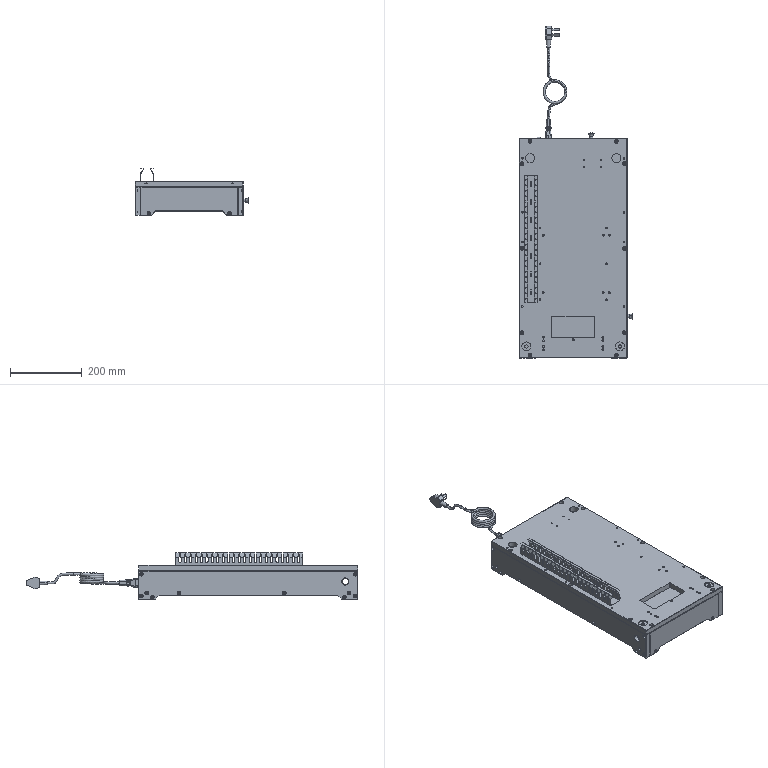Part | SolidWorks | 18 solids | 1893 faces | box 316 x 923.1 x 130.5 mm | volume 5362274 mm3 | plane 1006 | cylinder 750 | cone 76 | spline 61 | commonest cylinder face diameters 6 x180 5 x86 1 x78 4.2 x76 2 x73 10 x60